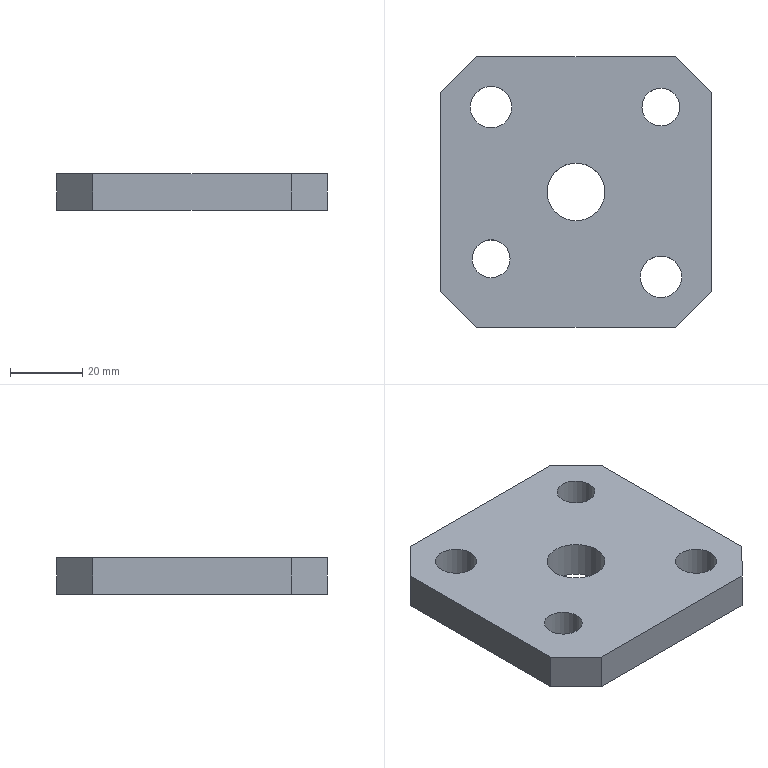Part | NX | features 23 2 | 1 solid | 15 faces | box 75 x 75 x 10 mm | volume 48427 mm3 | plane 10 | cylinder 5 | commonest cylinder face diameters 10.5 x2 11.509 x2 16 x1
STEP:
#1=CARTESIAN_POINT('',(13.306,0.,-33.5));
#2=VERTEX_POINT('',#1);
#3=CARTESIAN_POINT('',(21.306,0.,-33.5));
#4=DIRECTION('',(0.,0.,1.));
#5=DIRECTION('',(-1.,0.,0.));
#6=AXIS2_PLACEMENT_3D('',#3,#4,#5);
#7=CIRCLE('',#6,8.);
#8=EDGE_CURVE('',#2,#2,#7,.T.);
#9=ORIENTED_EDGE('',*,*,#8,.T.);
#10=EDGE_LOOP('',(#9));
#11=FACE_BOUND('',#10,.T.);
#12=CARTESIAN_POINT('',(13.306,0.,-43.5));
#13=VERTEX_POINT('',#12);
#14=CARTESIAN_POINT('',(21.306,0.,-43.5));
#15=DIRECTION('',(0.,0.,1.));
#16=DIRECTION('',(-1.,0.,0.));
#17=AXIS2_PLACEMENT_3D('',#14,#15,#16);
#18=CIRCLE('',#17,8.);
#19=EDGE_CURVE('',#13,#13,#18,.T.);
#20=ORIENTED_EDGE('',*,*,#19,.F.);
#21=EDGE_LOOP('',(#20));
#22=FACE_BOUND('',#21,.T.);
#23=CARTESIAN_POINT('',(21.306,0.,-33.5));
#24=DIRECTION('',(0.,0.,1.));
#25=DIRECTION('',(1.,0.,0.));
#26=AXIS2_PLACEMENT_3D('',#23,#24,#25);
#27=CYLINDRICAL_SURFACE('',#26,8.);
#28=ADVANCED_FACE('',(#11,#22),#27,.F.);
#29=CARTESIAN_POINT('',(-16.194,27.5,-33.5));
#30=VERTEX_POINT('',#29);
#31=CARTESIAN_POINT('',(-16.194,-27.5,-33.5));
#32=VERTEX_POINT('',#31);
#33=CARTESIAN_POINT('',(-16.194,0.,-33.5));
#34=DIRECTION('',(0.,-1.,0.));
#35=VECTOR('',#34,1000.);
#36=LINE('',#33,#35);
#37=EDGE_CURVE('',#30,#32,#36,.T.);
#38=ORIENTED_EDGE('',*,*,#37,.F.);
#39=CARTESIAN_POINT('',(-16.194,27.5,-43.5));
#40=VERTEX_POINT('',#39);
#41=CARTESIAN_POINT('',(-16.194,27.5,-33.5));
#42=DIRECTION('',(0.,0.,-1.));
#43=VECTOR('',#42,1000.);
#44=LINE('',#41,#43);
#45=EDGE_CURVE('',#30,#40,#44,.T.);
#46=ORIENTED_EDGE('',*,*,#45,.T.);
#47=CARTESIAN_POINT('',(-16.194,-27.5,-43.5));
#48=VERTEX_POINT('',#47);
#49=CARTESIAN_POINT('',(-16.194,-34.444,-43.5));
#50=DIRECTION('',(0.,-1.,0.));
#51=VECTOR('',#50,1000.);
#52=LINE('',#49,#51);
#53=EDGE_CURVE('',#40,#48,#52,.T.);
#54=ORIENTED_EDGE('',*,*,#53,.T.);
#55=CARTESIAN_POINT('',(-16.194,-27.5,-33.5));
#56=DIRECTION('',(0.,0.,1.));
#57=VECTOR('',#56,1000.);
#58=LINE('',#55,#57);
#59=EDGE_CURVE('',#48,#32,#58,.T.);
#60=ORIENTED_EDGE('',*,*,#59,.T.);
#61=EDGE_LOOP('',(#38,#46,#54,#60));
#62=FACE_BOUND('',#61,.T.);
#63=CARTESIAN_POINT('',(-16.194,0.,-33.5));
#64=DIRECTION('',(1.,0.,0.));
#65=DIRECTION('',(0.,-1.,0.));
#66=AXIS2_PLACEMENT_3D('',#63,#64,#65);
#67=PLANE('',#66);
#68=ADVANCED_FACE('',(#62),#67,.F.);
#69=CARTESIAN_POINT('',(48.806,37.5,-33.5));
#70=VERTEX_POINT('',#69);
#71=CARTESIAN_POINT('',(-6.194,37.5,-33.5));
#72=VERTEX_POINT('',#71);
#73=CARTESIAN_POINT('',(21.306,37.5,-33.5));
#74=DIRECTION('',(-1.,0.,0.));
#75=VECTOR('',#74,1000.);
#76=LINE('',#73,#75);
#77=EDGE_CURVE('',#70,#72,#76,.T.);
#78=ORIENTED_EDGE('',*,*,#77,.F.);
#79=CARTESIAN_POINT('',(48.806,37.5,-43.5));
#80=VERTEX_POINT('',#79);
#81=CARTESIAN_POINT('',(48.806,37.5,-33.5));
#82=DIRECTION('',(0.,0.,-1.));
#83=VECTOR('',#82,1000.);
#84=LINE('',#81,#83);
#85=EDGE_CURVE('',#70,#80,#84,.T.);
#86=ORIENTED_EDGE('',*,*,#85,.T.);
#87=CARTESIAN_POINT('',(-6.194,37.5,-43.5));
#88=VERTEX_POINT('',#87);
#89=CARTESIAN_POINT('',(53.733,37.5,-43.5));
#90=DIRECTION('',(-1.,0.,0.));
#91=VECTOR('',#90,1000.);
#92=LINE('',#89,#91);
#93=EDGE_CURVE('',#80,#88,#92,.T.);
#94=ORIENTED_EDGE('',*,*,#93,.T.);
#95=CARTESIAN_POINT('',(-6.194,37.5,-33.5));
#96=DIRECTION('',(0.,0.,1.));
#97=VECTOR('',#96,1000.);
#98=LINE('',#95,#97);
#99=EDGE_CURVE('',#88,#72,#98,.T.);
#100=ORIENTED_EDGE('',*,*,#99,.T.);
#101=EDGE_LOOP('',(#78,#86,#94,#100));
#102=FACE_BOUND('',#101,.T.);
#103=CARTESIAN_POINT('',(21.306,37.5,-33.5));
#104=DIRECTION('',(0.,-1.,0.));
#105=DIRECTION('',(-1.,0.,0.));
#106=AXIS2_PLACEMENT_3D('',#103,#104,#105);
#107=PLANE('',#106);
#108=ADVANCED_FACE('',(#102),#107,.F.);
#109=CARTESIAN_POINT('',(58.806,-27.5,-33.5));
#110=VERTEX_POINT('',#109);
#111=CARTESIAN_POINT('',(58.806,27.5,-33.5));
#112=VERTEX_POINT('',#111);
#113=CARTESIAN_POINT('',(58.806,0.,-33.5));
#114=DIRECTION('',(0.,1.,0.));
#115=VECTOR('',#114,1000.);
#116=LINE('',#113,#115);
#117=EDGE_CURVE('',#110,#112,#116,.T.);
#118=ORIENTED_EDGE('',*,*,#117,.F.);
#119=CARTESIAN_POINT('',(58.806,-27.5,-43.5));
#120=VERTEX_POINT('',#119);
#121=CARTESIAN_POINT('',(58.806,-27.5,-33.5));
#122=DIRECTION('',(0.,0.,-1.));
#123=VECTOR('',#122,1000.);
#124=LINE('',#121,#123);
#125=EDGE_CURVE('',#110,#120,#124,.T.);
#126=ORIENTED_EDGE('',*,*,#125,.T.);
#127=CARTESIAN_POINT('',(58.806,27.5,-43.5));
#128=VERTEX_POINT('',#127);
#129=CARTESIAN_POINT('',(58.806,-34.444,-43.5));
#130=DIRECTION('',(0.,1.,0.));
#131=VECTOR('',#130,1000.);
#132=LINE('',#129,#131);
#133=EDGE_CURVE('',#120,#128,#132,.T.);
#134=ORIENTED_EDGE('',*,*,#133,.T.);
#135=CARTESIAN_POINT('',(58.806,27.5,-33.5));
#136=DIRECTION('',(0.,0.,1.));
#137=VECTOR('',#136,1000.);
#138=LINE('',#135,#137);
#139=EDGE_CURVE('',#128,#112,#138,.T.);
#140=ORIENTED_EDGE('',*,*,#139,.T.);
#141=EDGE_LOOP('',(#118,#126,#134,#140));
#142=FACE_BOUND('',#141,.T.);
#143=CARTESIAN_POINT('',(58.806,0.,-33.5));
#144=DIRECTION('',(-1.,0.,0.));
#145=DIRECTION('',(0.,1.,0.));
#146=AXIS2_PLACEMENT_3D('',#143,#144,#145);
#147=PLANE('',#146);
#148=ADVANCED_FACE('',(#142),#147,.F.);
#149=CARTESIAN_POINT('',(-7.444,-18.5,-43.5));
#150=VERTEX_POINT('',#149);
#151=CARTESIAN_POINT('',(-2.194,-18.5,-43.5));
#152=DIRECTION('',(0.,0.,-1.));
#153=DIRECTION('',(-1.,0.,0.));
#154=AXIS2_PLACEMENT_3D('',#151,#152,#153);
#155=CIRCLE('',#154,5.25);
#156=EDGE_CURVE('',#150,#150,#155,.T.);
#157=ORIENTED_EDGE('',*,*,#156,.T.);
#158=EDGE_LOOP('',(#157));
#159=FACE_BOUND('',#158,.T.);
#160=CARTESIAN_POINT('',(-7.444,-18.5,-33.5));
#161=VERTEX_POINT('',#160);
#162=CARTESIAN_POINT('',(-2.194,-18.5,-33.5));
#163=DIRECTION('',(0.,0.,-1.));
#164=DIRECTION('',(-1.,0.,0.));
#165=AXIS2_PLACEMENT_3D('',#162,#163,#164);
#166=CIRCLE('',#165,5.25);
#167=EDGE_CURVE('',#161,#161,#166,.T.);
#168=ORIENTED_EDGE('',*,*,#167,.F.);
#169=EDGE_LOOP('',(#168));
#170=FACE_BOUND('',#169,.T.);
#171=CARTESIAN_POINT('',(-2.194,-18.5,-33.5));
#172=DIRECTION('',(0.,0.,-1.));
#173=DIRECTION('',(-1.,0.,0.));
#174=AXIS2_PLACEMENT_3D('',#171,#172,#173);
#175=CYLINDRICAL_SURFACE('',#174,5.25);
#176=ADVANCED_FACE('',(#159,#170),#175,.F.);
#177=CARTESIAN_POINT('',(-7.948,23.5,-43.5));
#178=VERTEX_POINT('',#177);
#179=CARTESIAN_POINT('',(-2.194,23.5,-43.5));
#180=DIRECTION('',(0.,0.,-1.));
#181=DIRECTION('',(-1.,0.,0.));
#182=AXIS2_PLACEMENT_3D('',#179,#180,#181);
#183=CIRCLE('',#182,5.755);
#184=EDGE_CURVE('',#178,#178,#183,.T.);
#185=ORIENTED_EDGE('',*,*,#184,.T.);
#186=EDGE_LOOP('',(#185));
#187=FACE_BOUND('',#186,.T.);
#188=CARTESIAN_POINT('',(-7.948,23.5,-33.5));
#189=VERTEX_POINT('',#188);
#190=CARTESIAN_POINT('',(-2.194,23.5,-33.5));
#191=DIRECTION('',(0.,0.,-1.));
#192=DIRECTION('',(-1.,0.,0.));
#193=AXIS2_PLACEMENT_3D('',#190,#191,#192);
#194=CIRCLE('',#193,5.755);
#195=EDGE_CURVE('',#189,#189,#194,.T.);
#196=ORIENTED_EDGE('',*,*,#195,.F.);
#197=EDGE_LOOP('',(#196));
#198=FACE_BOUND('',#197,.T.);
#199=CARTESIAN_POINT('',(-2.194,23.5,-33.5));
#200=DIRECTION('',(0.,0.,-1.));
#201=DIRECTION('',(-1.,0.,0.));
#202=AXIS2_PLACEMENT_3D('',#199,#200,#201);
#203=CYLINDRICAL_SURFACE('',#202,5.755);
#204=ADVANCED_FACE('',(#187,#198),#203,.F.);
#205=CARTESIAN_POINT('',(39.556,23.5,-43.5));
#206=VERTEX_POINT('',#205);
#207=CARTESIAN_POINT('',(44.806,23.5,-43.5));
#208=DIRECTION('',(0.,0.,-1.));
#209=DIRECTION('',(-1.,0.,0.));
#210=AXIS2_PLACEMENT_3D('',#207,#208,#209);
#211=CIRCLE('',#210,5.25);
#212=EDGE_CURVE('',#206,#206,#211,.T.);
#213=ORIENTED_EDGE('',*,*,#212,.T.);
#214=EDGE_LOOP('',(#213));
#215=FACE_BOUND('',#214,.T.);
#216=CARTESIAN_POINT('',(39.556,23.5,-33.5));
#217=VERTEX_POINT('',#216);
#218=CARTESIAN_POINT('',(44.806,23.5,-33.5));
#219=DIRECTION('',(0.,0.,-1.));
#220=DIRECTION('',(-1.,0.,0.));
#221=AXIS2_PLACEMENT_3D('',#218,#219,#220);
#222=CIRCLE('',#221,5.25);
#223=EDGE_CURVE('',#217,#217,#222,.T.);
#224=ORIENTED_EDGE('',*,*,#223,.F.);
#225=EDGE_LOOP('',(#224));
#226=FACE_BOUND('',#225,.T.);
#227=CARTESIAN_POINT('',(44.806,23.5,-33.5));
#228=DIRECTION('',(0.,0.,-1.));
#229=DIRECTION('',(-1.,0.,0.));
#230=AXIS2_PLACEMENT_3D('',#227,#228,#229);
#231=CYLINDRICAL_SURFACE('',#230,5.25);
#232=ADVANCED_FACE('',(#215,#226),#231,.F.);
#233=CARTESIAN_POINT('',(39.052,-23.5,-43.5));
#234=VERTEX_POINT('',#233);
#235=CARTESIAN_POINT('',(44.806,-23.5,-43.5));
#236=DIRECTION('',(0.,0.,-1.));
#237=DIRECTION('',(-1.,0.,0.));
#238=AXIS2_PLACEMENT_3D('',#235,#236,#237);
#239=CIRCLE('',#238,5.755);
#240=EDGE_CURVE('',#234,#234,#239,.T.);
#241=ORIENTED_EDGE('',*,*,#240,.T.);
#242=EDGE_LOOP('',(#241));
#243=FACE_BOUND('',#242,.T.);
#244=CARTESIAN_POINT('',(39.052,-23.5,-33.5));
#245=VERTEX_POINT('',#244);
#246=CARTESIAN_POINT('',(44.806,-23.5,-33.5));
#247=DIRECTION('',(0.,0.,-1.));
#248=DIRECTION('',(-1.,0.,0.));
#249=AXIS2_PLACEMENT_3D('',#246,#247,#248);
#250=CIRCLE('',#249,5.755);
#251=EDGE_CURVE('',#245,#245,#250,.T.);
#252=ORIENTED_EDGE('',*,*,#251,.F.);
#253=EDGE_LOOP('',(#252));
#254=FACE_BOUND('',#253,.T.);
#255=CARTESIAN_POINT('',(44.806,-23.5,-33.5));
#256=DIRECTION('',(0.,0.,-1.));
#257=DIRECTION('',(-1.,0.,0.));
#258=AXIS2_PLACEMENT_3D('',#255,#256,#257);
#259=CYLINDRICAL_SURFACE('',#258,5.755);
#260=ADVANCED_FACE('',(#243,#254),#259,.F.);
#261=CARTESIAN_POINT('',(-6.194,-37.5,-43.5));
#262=VERTEX_POINT('',#261);
#263=CARTESIAN_POINT('',(48.806,-37.5,-43.5));
#264=VERTEX_POINT('',#263);
#265=CARTESIAN_POINT('',(53.733,-37.5,-43.5));
#266=DIRECTION('',(1.,0.,0.));
#267=VECTOR('',#266,1000.);
#268=LINE('',#265,#267);
#269=EDGE_CURVE('',#262,#264,#268,.T.);
#270=ORIENTED_EDGE('',*,*,#269,.T.);
#271=CARTESIAN_POINT('',(48.806,-37.5,-33.5));
#272=VERTEX_POINT('',#271);
#273=CARTESIAN_POINT('',(48.806,-37.5,-33.5));
#274=DIRECTION('',(0.,0.,1.));
#275=VECTOR('',#274,1000.);
#276=LINE('',#273,#275);
#277=EDGE_CURVE('',#264,#272,#276,.T.);
#278=ORIENTED_EDGE('',*,*,#277,.T.);
#279=CARTESIAN_POINT('',(-6.194,-37.5,-33.5));
#280=VERTEX_POINT('',#279);
#281=CARTESIAN_POINT('',(21.306,-37.5,-33.5));
#282=DIRECTION('',(1.,0.,0.));
#283=VECTOR('',#282,1000.);
#284=LINE('',#281,#283);
#285=EDGE_CURVE('',#280,#272,#284,.T.);
#286=ORIENTED_EDGE('',*,*,#285,.F.);
#287=CARTESIAN_POINT('',(-6.194,-37.5,-33.5));
#288=DIRECTION('',(0.,0.,-1.));
#289=VECTOR('',#288,1000.);
#290=LINE('',#287,#289);
#291=EDGE_CURVE('',#280,#262,#290,.T.);
#292=ORIENTED_EDGE('',*,*,#291,.T.);
#293=EDGE_LOOP('',(#270,#278,#286,#292));
#294=FACE_BOUND('',#293,.T.);
#295=CARTESIAN_POINT('',(21.306,-37.5,-33.5));
#296=DIRECTION('',(0.,1.,0.));
#297=DIRECTION('',(1.,0.,0.));
#298=AXIS2_PLACEMENT_3D('',#295,#296,#297);
#299=PLANE('',#298);
#300=ADVANCED_FACE('',(#294),#299,.F.);
#301=ORIENTED_EDGE('',*,*,#156,.F.);
#302=EDGE_LOOP('',(#301));
#303=FACE_BOUND('',#302,.T.);
#304=ORIENTED_EDGE('',*,*,#184,.F.);
#305=EDGE_LOOP('',(#304));
#306=FACE_BOUND('',#305,.T.);
#307=ORIENTED_EDGE('',*,*,#212,.F.);
#308=EDGE_LOOP('',(#307));
#309=FACE_BOUND('',#308,.T.);
#310=ORIENTED_EDGE('',*,*,#240,.F.);
#311=EDGE_LOOP('',(#310));
#312=FACE_BOUND('',#311,.T.);
#313=ORIENTED_EDGE('',*,*,#133,.F.);
#314=CARTESIAN_POINT('',(55.297,-31.009,-43.5));
#315=DIRECTION('',(-0.7071,-0.7071,0.));
#316=VECTOR('',#315,1000.);
#317=LINE('',#314,#316);
#318=EDGE_CURVE('',#120,#264,#317,.T.);
#319=ORIENTED_EDGE('',*,*,#318,.T.);
#320=ORIENTED_EDGE('',*,*,#269,.F.);
#321=CARTESIAN_POINT('',(19.741,-63.435,-43.5));
#322=DIRECTION('',(-0.7071,0.7071,0.));
#323=VECTOR('',#322,1000.);
#324=LINE('',#321,#323);
#325=EDGE_CURVE('',#262,#48,#324,.T.);
#326=ORIENTED_EDGE('',*,*,#325,.T.);
#327=ORIENTED_EDGE('',*,*,#53,.F.);
#328=CARTESIAN_POINT('',(-14.703,28.991,-43.5));
#329=DIRECTION('',(0.7071,0.7071,0.));
#330=VECTOR('',#329,1000.);
#331=LINE('',#328,#330);
#332=EDGE_CURVE('',#40,#88,#331,.T.);
#333=ORIENTED_EDGE('',*,*,#332,.T.);
#334=ORIENTED_EDGE('',*,*,#93,.F.);
#335=CARTESIAN_POINT('',(89.741,-3.435,-43.5));
#336=DIRECTION('',(0.7071,-0.7071,0.));
#337=VECTOR('',#336,1000.);
#338=LINE('',#335,#337);
#339=EDGE_CURVE('',#80,#128,#338,.T.);
#340=ORIENTED_EDGE('',*,*,#339,.T.);
#341=EDGE_LOOP('',(#313,#319,#320,#326,#327,#333,#334,#340));
#342=FACE_BOUND('',#341,.T.);
#343=ORIENTED_EDGE('',*,*,#19,.T.);
#344=EDGE_LOOP('',(#343));
#345=FACE_BOUND('',#344,.T.);
#346=CARTESIAN_POINT('',(53.733,-34.444,-43.5));
#347=DIRECTION('',(0.,0.,-1.));
#348=DIRECTION('',(-1.,0.,0.));
#349=AXIS2_PLACEMENT_3D('',#346,#347,#348);
#350=PLANE('',#349);
#351=ADVANCED_FACE('',(#303,#306,#309,#312,#342,#345),#350,.T.);
#352=ORIENTED_EDGE('',*,*,#167,.T.);
#353=EDGE_LOOP('',(#352));
#354=FACE_BOUND('',#353,.T.);
#355=ORIENTED_EDGE('',*,*,#195,.T.);
#356=EDGE_LOOP('',(#355));
#357=FACE_BOUND('',#356,.T.);
#358=ORIENTED_EDGE('',*,*,#223,.T.);
#359=EDGE_LOOP('',(#358));
#360=FACE_BOUND('',#359,.T.);
#361=ORIENTED_EDGE('',*,*,#251,.T.);
#362=EDGE_LOOP('',(#361));
#363=FACE_BOUND('',#362,.T.);
#364=ORIENTED_EDGE('',*,*,#285,.T.);
#365=CARTESIAN_POINT('',(58.806,-27.5,-33.5));
#366=DIRECTION('',(0.7071,0.7071,0.));
#367=VECTOR('',#366,1000.);
#368=LINE('',#365,#367);
#369=EDGE_CURVE('',#272,#110,#368,.T.);
#370=ORIENTED_EDGE('',*,*,#369,.T.);
#371=ORIENTED_EDGE('',*,*,#117,.T.);
#372=CARTESIAN_POINT('',(53.806,32.5,-33.5));
#373=DIRECTION('',(-0.7071,0.7071,0.));
#374=VECTOR('',#373,1000.);
#375=LINE('',#372,#374);
#376=EDGE_CURVE('',#112,#70,#375,.T.);
#377=ORIENTED_EDGE('',*,*,#376,.T.);
#378=ORIENTED_EDGE('',*,*,#77,.T.);
#379=CARTESIAN_POINT('',(-16.194,27.5,-33.5));
#380=DIRECTION('',(-0.7071,-0.7071,0.));
#381=VECTOR('',#380,1000.);
#382=LINE('',#379,#381);
#383=EDGE_CURVE('',#72,#30,#382,.T.);
#384=ORIENTED_EDGE('',*,*,#383,.T.);
#385=ORIENTED_EDGE('',*,*,#37,.T.);
#386=CARTESIAN_POINT('',(-11.194,-32.5,-33.5));
#387=DIRECTION('',(0.7071,-0.7071,0.));
#388=VECTOR('',#387,1000.);
#389=LINE('',#386,#388);
#390=EDGE_CURVE('',#32,#280,#389,.T.);
#391=ORIENTED_EDGE('',*,*,#390,.T.);
#392=EDGE_LOOP('',(#364,#370,#371,#377,#378,#384,#385,#391));
#393=FACE_BOUND('',#392,.T.);
#394=ORIENTED_EDGE('',*,*,#8,.F.);
#395=EDGE_LOOP('',(#394));
#396=FACE_BOUND('',#395,.T.);
#397=CARTESIAN_POINT('',(53.733,-34.444,-33.5));
#398=DIRECTION('',(0.,0.,-1.));
#399=DIRECTION('',(-1.,0.,0.));
#400=AXIS2_PLACEMENT_3D('',#397,#398,#399);
#401=PLANE('',#400);
#402=ADVANCED_FACE('',(#354,#357,#360,#363,#393,#396),#401,.F.);
#403=ORIENTED_EDGE('',*,*,#369,.F.);
#404=ORIENTED_EDGE('',*,*,#277,.F.);
#405=ORIENTED_EDGE('',*,*,#318,.F.);
#406=ORIENTED_EDGE('',*,*,#125,.F.);
#407=EDGE_LOOP('',(#403,#404,#405,#406));
#408=FACE_BOUND('',#407,.T.);
#409=CARTESIAN_POINT('',(58.806,-27.5,-33.5));
#410=DIRECTION('',(-0.7071,0.7071,0.));
#411=DIRECTION('',(0.,0.,-1.));
#412=AXIS2_PLACEMENT_3D('',#409,#410,#411);
#413=PLANE('',#412);
#414=ADVANCED_FACE('',(#408),#413,.F.);
#415=ORIENTED_EDGE('',*,*,#376,.F.);
#416=ORIENTED_EDGE('',*,*,#139,.F.);
#417=ORIENTED_EDGE('',*,*,#339,.F.);
#418=ORIENTED_EDGE('',*,*,#85,.F.);
#419=EDGE_LOOP('',(#415,#416,#417,#418));
#420=FACE_BOUND('',#419,.T.);
#421=CARTESIAN_POINT('',(53.806,32.5,-33.5));
#422=DIRECTION('',(-0.7071,-0.7071,0.));
#423=DIRECTION('',(0.,0.,-1.));
#424=AXIS2_PLACEMENT_3D('',#421,#422,#423);
#425=PLANE('',#424);
#426=ADVANCED_FACE('',(#420),#425,.F.);
#427=ORIENTED_EDGE('',*,*,#383,.F.);
#428=ORIENTED_EDGE('',*,*,#99,.F.);
#429=ORIENTED_EDGE('',*,*,#332,.F.);
#430=ORIENTED_EDGE('',*,*,#45,.F.);
#431=EDGE_LOOP('',(#427,#428,#429,#430));
#432=FACE_BOUND('',#431,.T.);
#433=CARTESIAN_POINT('',(-16.194,27.5,-33.5));
#434=DIRECTION('',(0.7071,-0.7071,0.));
#435=DIRECTION('',(0.,0.,-1.));
#436=AXIS2_PLACEMENT_3D('',#433,#434,#435);
#437=PLANE('',#436);
#438=ADVANCED_FACE('',(#432),#437,.F.);
#439=ORIENTED_EDGE('',*,*,#390,.F.);
#440=ORIENTED_EDGE('',*,*,#59,.F.);
#441=ORIENTED_EDGE('',*,*,#325,.F.);
#442=ORIENTED_EDGE('',*,*,#291,.F.);
#443=EDGE_LOOP('',(#439,#440,#441,#442));
#444=FACE_BOUND('',#443,.T.);
#445=CARTESIAN_POINT('',(-11.194,-32.5,-33.5));
#446=DIRECTION('',(0.7071,0.7071,0.));
#447=DIRECTION('',(0.,0.,-1.));
#448=AXIS2_PLACEMENT_3D('',#445,#446,#447);
#449=PLANE('',#448);
#450=ADVANCED_FACE('',(#444),#449,.F.);
#451=CLOSED_SHELL('',(#28,#68,#108,#148,#176,#204,#232,#260,#300,#351,#402,#414,#426,#438,#450));
#452=MANIFOLD_SOLID_BREP('',#451);
#453=(LENGTH_UNIT()NAMED_UNIT(*)SI_UNIT(.MILLI.,.METRE.));
#454=UNCERTAINTY_MEASURE_WITH_UNIT(LENGTH_MEASURE(0.00001),#453,'','');
#455=(NAMED_UNIT(*)PLANE_ANGLE_UNIT()SI_UNIT($,.RADIAN.));
#456=(NAMED_UNIT(*)SI_UNIT($,.STERADIAN.)SOLID_ANGLE_UNIT());
#457=(GEOMETRIC_REPRESENTATION_CONTEXT(3)GLOBAL_UNCERTAINTY_ASSIGNED_CONTEXT((#454))GLOBAL_UNIT_ASSIGNED_CONTEXT((#453,#455,#456))REPRESENTATION_CONTEXT('',''));
#458=ADVANCED_BREP_SHAPE_REPRESENTATION('',(#452),#457);